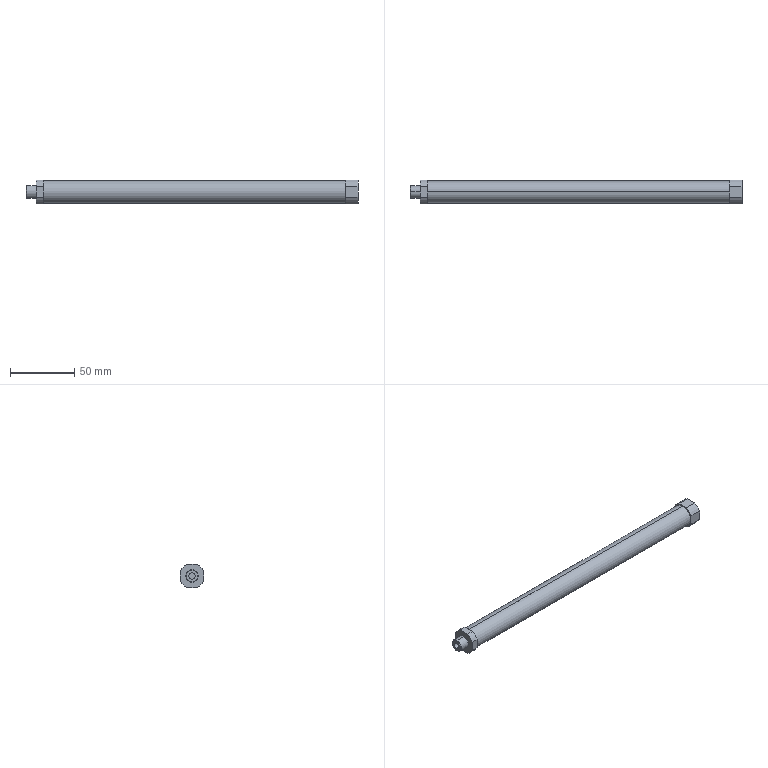Part | SolidWorks | features Chamfer 2, HoleWzd 2, ICE 2, Extrusion 1, Revolution 1 | 1 solid | 39 faces | box 259 x 18.3 x 18.3 mm | volume 34694 mm3 | cylinder 18 | plane 15 | cone 6 | commonest cylinder face diameters 20 x8 4.134 x2 5 x2 10 x2 16 x2 17.4 x2
STEP:
#1=CARTESIAN_POINT('',(246.,8.717,-2.067));
#2=VERTEX_POINT('',#1);
#3=CARTESIAN_POINT('',(246.,8.717,2.067));
#4=VERTEX_POINT('',#3);
#5=CARTESIAN_POINT('',(246.,8.717,0.));
#6=DIRECTION('',(0.,1.,0.));
#7=DIRECTION('',(0.,0.,1.));
#8=AXIS2_PLACEMENT_3D('',#5,#6,#7);
#9=CIRCLE('',#8,2.067);
#10=EDGE_CURVE('',#2,#4,#9,.T.);
#11=ORIENTED_EDGE('',*,*,#10,.F.);
#12=CARTESIAN_POINT('',(246.,9.15,-2.5));
#13=VERTEX_POINT('',#12);
#14=CARTESIAN_POINT('',(246.,8.717,-2.067));
#15=DIRECTION('',(0.,0.7071,-0.7071));
#16=VECTOR('',#15,1000.);
#17=LINE('',#14,#16);
#18=EDGE_CURVE('',#2,#13,#17,.T.);
#19=ORIENTED_EDGE('',*,*,#18,.T.);
#20=CARTESIAN_POINT('',(246.,9.15,2.5));
#21=VERTEX_POINT('',#20);
#22=CARTESIAN_POINT('',(246.,9.15,0.));
#23=DIRECTION('',(0.,-1.,0.));
#24=DIRECTION('',(0.,0.,1.));
#25=AXIS2_PLACEMENT_3D('',#22,#23,#24);
#26=CIRCLE('',#25,2.5);
#27=EDGE_CURVE('',#21,#13,#26,.T.);
#28=ORIENTED_EDGE('',*,*,#27,.F.);
#29=CARTESIAN_POINT('',(246.,8.717,2.067));
#30=DIRECTION('',(0.,0.7071,0.7071));
#31=VECTOR('',#30,1000.);
#32=LINE('',#29,#31);
#33=EDGE_CURVE('',#4,#21,#32,.T.);
#34=ORIENTED_EDGE('',*,*,#33,.F.);
#35=EDGE_LOOP('',(#11,#19,#28,#34));
#36=FACE_OUTER_BOUND('',#35,.T.);
#37=CARTESIAN_POINT('',(246.,8.717,0.));
#38=DIRECTION('',(0.,1.,0.));
#39=DIRECTION('',(0.,0.,1.));
#40=AXIS2_PLACEMENT_3D('',#37,#38,#39);
#41=CONICAL_SURFACE('',#40,2.067,0.7854);
#42=ADVANCED_FACE('',(#36),#41,.F.);
#43=CARTESIAN_POINT('',(-8.,0.,4.459));
#44=VERTEX_POINT('',#43);
#45=CARTESIAN_POINT('',(-8.,0.,-4.459));
#46=VERTEX_POINT('',#45);
#47=CARTESIAN_POINT('',(-8.,0.,0.));
#48=DIRECTION('',(-1.,0.,0.));
#49=DIRECTION('',(0.,0.,1.));
#50=AXIS2_PLACEMENT_3D('',#47,#48,#49);
#51=CIRCLE('',#50,4.459);
#52=EDGE_CURVE('',#44,#46,#51,.T.);
#53=ORIENTED_EDGE('',*,*,#52,.F.);
#54=CARTESIAN_POINT('',(-7.459,0.,5.));
#55=VERTEX_POINT('',#54);
#56=CARTESIAN_POINT('',(-7.459,0.,5.));
#57=DIRECTION('',(0.7071,0.,0.7071));
#58=VECTOR('',#57,1000.);
#59=LINE('',#56,#58);
#60=EDGE_CURVE('',#44,#55,#59,.T.);
#61=ORIENTED_EDGE('',*,*,#60,.T.);
#62=CARTESIAN_POINT('',(-7.459,0.,-5.));
#63=VERTEX_POINT('',#62);
#64=CARTESIAN_POINT('',(-7.459,0.,0.));
#65=DIRECTION('',(1.,0.,0.));
#66=DIRECTION('',(0.,0.,1.));
#67=AXIS2_PLACEMENT_3D('',#64,#65,#66);
#68=CIRCLE('',#67,5.);
#69=EDGE_CURVE('',#63,#55,#68,.T.);
#70=ORIENTED_EDGE('',*,*,#69,.F.);
#71=CARTESIAN_POINT('',(-7.459,0.,-5.));
#72=DIRECTION('',(0.7071,0.,-0.7071));
#73=VECTOR('',#72,1000.);
#74=LINE('',#71,#73);
#75=EDGE_CURVE('',#46,#63,#74,.T.);
#76=ORIENTED_EDGE('',*,*,#75,.F.);
#77=EDGE_LOOP('',(#53,#61,#70,#76));
#78=FACE_OUTER_BOUND('',#77,.T.);
#79=CARTESIAN_POINT('',(-7.459,0.,0.));
#80=DIRECTION('',(1.,0.,0.));
#81=DIRECTION('',(0.,0.,-1.));
#82=AXIS2_PLACEMENT_3D('',#79,#80,#81);
#83=CONICAL_SURFACE('',#82,5.,0.7854);
#84=ADVANCED_FACE('',(#78),#83,.T.);
#85=CARTESIAN_POINT('',(5.5,0.,-2.5));
#86=VERTEX_POINT('',#85);
#87=CARTESIAN_POINT('',(5.5,0.,2.5));
#88=VERTEX_POINT('',#87);
#89=CARTESIAN_POINT('',(5.5,0.,0.));
#90=DIRECTION('',(-1.,0.,0.));
#91=DIRECTION('',(0.,0.,1.));
#92=AXIS2_PLACEMENT_3D('',#89,#90,#91);
#93=CIRCLE('',#92,2.5);
#94=EDGE_CURVE('',#86,#88,#93,.T.);
#95=ORIENTED_EDGE('',*,*,#94,.F.);
#96=CARTESIAN_POINT('',(-8.,0.,-2.5));
#97=VERTEX_POINT('',#96);
#98=CARTESIAN_POINT('',(-8.,0.,-2.5));
#99=DIRECTION('',(-1.,0.,0.));
#100=VECTOR('',#99,1000.);
#101=LINE('',#98,#100);
#102=EDGE_CURVE('',#86,#97,#101,.T.);
#103=ORIENTED_EDGE('',*,*,#102,.T.);
#104=CARTESIAN_POINT('',(-8.,0.,2.5));
#105=VERTEX_POINT('',#104);
#106=CARTESIAN_POINT('',(-8.,0.,0.));
#107=DIRECTION('',(-1.,0.,0.));
#108=DIRECTION('',(0.,0.,1.));
#109=AXIS2_PLACEMENT_3D('',#106,#107,#108);
#110=CIRCLE('',#109,2.5);
#111=EDGE_CURVE('',#97,#105,#110,.T.);
#112=ORIENTED_EDGE('',*,*,#111,.T.);
#113=CARTESIAN_POINT('',(-8.,0.,2.5));
#114=DIRECTION('',(-1.,0.,0.));
#115=VECTOR('',#114,1000.);
#116=LINE('',#113,#115);
#117=EDGE_CURVE('',#88,#105,#116,.T.);
#118=ORIENTED_EDGE('',*,*,#117,.F.);
#119=EDGE_LOOP('',(#95,#103,#112,#118));
#120=FACE_OUTER_BOUND('',#119,.T.);
#121=CARTESIAN_POINT('',(-8.,0.,0.));
#122=DIRECTION('',(-1.,0.,0.));
#123=DIRECTION('',(0.,0.,1.));
#124=AXIS2_PLACEMENT_3D('',#121,#122,#123);
#125=CYLINDRICAL_SURFACE('',#124,2.5);
#126=ADVANCED_FACE('',(#120),#125,.F.);
#127=CARTESIAN_POINT('',(135.5,0.,-8.));
#128=VERTEX_POINT('',#127);
#129=CARTESIAN_POINT('',(135.5,0.,8.));
#130=VERTEX_POINT('',#129);
#131=CARTESIAN_POINT('',(135.5,0.,0.));
#132=DIRECTION('',(-1.,0.,0.));
#133=DIRECTION('',(0.,0.,1.));
#134=AXIS2_PLACEMENT_3D('',#131,#132,#133);
#135=CIRCLE('',#134,8.);
#136=EDGE_CURVE('',#128,#130,#135,.T.);
#137=ORIENTED_EDGE('',*,*,#136,.F.);
#138=CARTESIAN_POINT('',(5.5,0.,-8.));
#139=VERTEX_POINT('',#138);
#140=CARTESIAN_POINT('',(-8.,0.,-8.));
#141=DIRECTION('',(-1.,0.,0.));
#142=VECTOR('',#141,1000.);
#143=LINE('',#140,#142);
#144=EDGE_CURVE('',#128,#139,#143,.T.);
#145=ORIENTED_EDGE('',*,*,#144,.T.);
#146=CARTESIAN_POINT('',(5.5,0.,8.));
#147=VERTEX_POINT('',#146);
#148=CARTESIAN_POINT('',(5.5,0.,0.));
#149=DIRECTION('',(-1.,0.,0.));
#150=DIRECTION('',(0.,0.,1.));
#151=AXIS2_PLACEMENT_3D('',#148,#149,#150);
#152=CIRCLE('',#151,8.);
#153=EDGE_CURVE('',#139,#147,#152,.T.);
#154=ORIENTED_EDGE('',*,*,#153,.T.);
#155=CARTESIAN_POINT('',(-8.,0.,8.));
#156=DIRECTION('',(-1.,0.,0.));
#157=VECTOR('',#156,1000.);
#158=LINE('',#155,#157);
#159=EDGE_CURVE('',#130,#147,#158,.T.);
#160=ORIENTED_EDGE('',*,*,#159,.F.);
#161=EDGE_LOOP('',(#137,#145,#154,#160));
#162=FACE_OUTER_BOUND('',#161,.T.);
#163=CARTESIAN_POINT('',(-8.,0.,0.));
#164=DIRECTION('',(-1.,0.,0.));
#165=DIRECTION('',(0.,0.,1.));
#166=AXIS2_PLACEMENT_3D('',#163,#164,#165);
#167=CYLINDRICAL_SURFACE('',#166,8.);
#168=ADVANCED_FACE('',(#162),#167,.F.);
#169=CARTESIAN_POINT('',(246.,3.65,-2.067));
#170=VERTEX_POINT('',#169);
#171=CARTESIAN_POINT('',(246.,3.65,2.067));
#172=VERTEX_POINT('',#171);
#173=CARTESIAN_POINT('',(246.,3.65,0.));
#174=DIRECTION('',(0.,1.,0.));
#175=DIRECTION('',(0.,0.,1.));
#176=AXIS2_PLACEMENT_3D('',#173,#174,#175);
#177=CIRCLE('',#176,2.067);
#178=EDGE_CURVE('',#170,#172,#177,.T.);
#179=ORIENTED_EDGE('',*,*,#178,.F.);
#180=CARTESIAN_POINT('',(246.,9.15,-2.067));
#181=DIRECTION('',(0.,1.,0.));
#182=VECTOR('',#181,1000.);
#183=LINE('',#180,#182);
#184=EDGE_CURVE('',#170,#2,#183,.T.);
#185=ORIENTED_EDGE('',*,*,#184,.T.);
#186=ORIENTED_EDGE('',*,*,#10,.T.);
#187=CARTESIAN_POINT('',(246.,9.15,2.067));
#188=DIRECTION('',(0.,1.,0.));
#189=VECTOR('',#188,1000.);
#190=LINE('',#187,#189);
#191=EDGE_CURVE('',#172,#4,#190,.T.);
#192=ORIENTED_EDGE('',*,*,#191,.F.);
#193=EDGE_LOOP('',(#179,#185,#186,#192));
#194=FACE_OUTER_BOUND('',#193,.T.);
#195=CARTESIAN_POINT('',(246.,9.15,0.));
#196=DIRECTION('',(0.,1.,0.));
#197=DIRECTION('',(0.,0.,1.));
#198=AXIS2_PLACEMENT_3D('',#195,#196,#197);
#199=CYLINDRICAL_SURFACE('',#198,2.067);
#200=ADVANCED_FACE('',(#194),#199,.F.);
#201=CARTESIAN_POINT('',(246.,2.457,0.));
#202=VERTEX_POINT('',#201);
#203=CARTESIAN_POINT('',(246.,3.65,2.067));
#204=DIRECTION('',(0.,0.5,0.866));
#205=VECTOR('',#204,1000.);
#206=LINE('',#203,#205);
#207=EDGE_CURVE('',#202,#172,#206,.T.);
#208=ORIENTED_EDGE('',*,*,#207,.F.);
#209=CARTESIAN_POINT('',(246.,3.65,-2.067));
#210=DIRECTION('',(0.,0.5,-0.866));
#211=VECTOR('',#210,1000.);
#212=LINE('',#209,#211);
#213=EDGE_CURVE('',#202,#170,#212,.T.);
#214=ORIENTED_EDGE('',*,*,#213,.T.);
#215=ORIENTED_EDGE('',*,*,#178,.T.);
#216=EDGE_LOOP('',(#208,#214,#215));
#217=FACE_OUTER_BOUND('',#216,.T.);
#218=CARTESIAN_POINT('',(246.,3.65,0.));
#219=DIRECTION('',(0.,1.,0.));
#220=DIRECTION('',(0.,0.,1.));
#221=AXIS2_PLACEMENT_3D('',#218,#219,#220);
#222=CONICAL_SURFACE('',#221,2.067,1.047);
#223=ADVANCED_FACE('',(#217),#222,.F.);
#224=ORIENTED_EDGE('',*,*,#69,.T.);
#225=CARTESIAN_POINT('',(0.,0.,5.));
#226=VERTEX_POINT('',#225);
#227=CARTESIAN_POINT('',(-8.,0.,5.));
#228=DIRECTION('',(1.,0.,0.));
#229=VECTOR('',#228,1000.);
#230=LINE('',#227,#229);
#231=EDGE_CURVE('',#55,#226,#230,.T.);
#232=ORIENTED_EDGE('',*,*,#231,.T.);
#233=CARTESIAN_POINT('',(0.,0.,-5.));
#234=VERTEX_POINT('',#233);
#235=CARTESIAN_POINT('',(0.,0.,0.));
#236=DIRECTION('',(-1.,0.,0.));
#237=DIRECTION('',(0.,0.,1.));
#238=AXIS2_PLACEMENT_3D('',#235,#236,#237);
#239=CIRCLE('',#238,5.);
#240=EDGE_CURVE('',#226,#234,#239,.T.);
#241=ORIENTED_EDGE('',*,*,#240,.T.);
#242=CARTESIAN_POINT('',(-8.,0.,-5.));
#243=DIRECTION('',(1.,0.,0.));
#244=VECTOR('',#243,1000.);
#245=LINE('',#242,#244);
#246=EDGE_CURVE('',#63,#234,#245,.T.);
#247=ORIENTED_EDGE('',*,*,#246,.F.);
#248=EDGE_LOOP('',(#224,#232,#241,#247));
#249=FACE_OUTER_BOUND('',#248,.T.);
#250=CARTESIAN_POINT('',(-8.,0.,0.));
#251=DIRECTION('',(1.,0.,0.));
#252=DIRECTION('',(0.,0.,-1.));
#253=AXIS2_PLACEMENT_3D('',#250,#251,#252);
#254=CYLINDRICAL_SURFACE('',#253,5.);
#255=ADVANCED_FACE('',(#249),#254,.T.);
#256=CARTESIAN_POINT('',(241.5,0.,-8.7));
#257=VERTEX_POINT('',#256);
#258=CARTESIAN_POINT('',(241.5,0.,8.7));
#259=VERTEX_POINT('',#258);
#260=CARTESIAN_POINT('',(241.5,0.,0.));
#261=DIRECTION('',(1.,0.,0.));
#262=DIRECTION('',(0.,0.,-1.));
#263=AXIS2_PLACEMENT_3D('',#260,#261,#262);
#264=CIRCLE('',#263,8.7);
#265=EDGE_CURVE('',#257,#259,#264,.T.);
#266=ORIENTED_EDGE('',*,*,#265,.F.);
#267=CARTESIAN_POINT('',(5.5,0.,-8.7));
#268=VERTEX_POINT('',#267);
#269=CARTESIAN_POINT('',(241.5,0.,-8.7));
#270=DIRECTION('',(-1.,0.,0.));
#271=VECTOR('',#270,1000.);
#272=LINE('',#269,#271);
#273=EDGE_CURVE('',#257,#268,#272,.T.);
#274=ORIENTED_EDGE('',*,*,#273,.T.);
#275=CARTESIAN_POINT('',(5.5,0.,8.7));
#276=VERTEX_POINT('',#275);
#277=CARTESIAN_POINT('',(5.5,0.,0.));
#278=DIRECTION('',(1.,0.,0.));
#279=DIRECTION('',(0.,0.,1.));
#280=AXIS2_PLACEMENT_3D('',#277,#278,#279);
#281=CIRCLE('',#280,8.7);
#282=EDGE_CURVE('',#268,#276,#281,.T.);
#283=ORIENTED_EDGE('',*,*,#282,.T.);
#284=CARTESIAN_POINT('',(241.5,0.,8.7));
#285=DIRECTION('',(-1.,0.,0.));
#286=VECTOR('',#285,1000.);
#287=LINE('',#284,#286);
#288=EDGE_CURVE('',#259,#276,#287,.T.);
#289=ORIENTED_EDGE('',*,*,#288,.F.);
#290=EDGE_LOOP('',(#266,#274,#283,#289));
#291=FACE_OUTER_BOUND('',#290,.T.);
#292=CARTESIAN_POINT('',(241.5,0.,0.));
#293=DIRECTION('',(-1.,0.,0.));
#294=DIRECTION('',(0.,0.,1.));
#295=AXIS2_PLACEMENT_3D('',#292,#293,#294);
#296=CYLINDRICAL_SURFACE('',#295,8.7);
#297=ADVANCED_FACE('',(#291),#296,.T.);
#298=CARTESIAN_POINT('',(5.5,-9.15,4.035));
#299=VERTEX_POINT('',#298);
#300=CARTESIAN_POINT('',(5.5,-4.035,9.15));
#301=VERTEX_POINT('',#300);
#302=CARTESIAN_POINT('',(5.5,0.,0.));
#303=DIRECTION('',(-1.,0.,0.));
#304=DIRECTION('',(0.,0.,1.));
#305=AXIS2_PLACEMENT_3D('',#302,#303,#304);
#306=CIRCLE('',#305,10.);
#307=EDGE_CURVE('',#299,#301,#306,.T.);
#308=ORIENTED_EDGE('',*,*,#307,.F.);
#309=CARTESIAN_POINT('',(5.5,-9.15,-4.035));
#310=VERTEX_POINT('',#309);
#311=CARTESIAN_POINT('',(5.5,-9.15,-4.035));
#312=DIRECTION('',(0.,0.,1.));
#313=VECTOR('',#312,1000.);
#314=LINE('',#311,#313);
#315=EDGE_CURVE('',#310,#299,#314,.T.);
#316=ORIENTED_EDGE('',*,*,#315,.F.);
#317=CARTESIAN_POINT('',(5.5,-4.035,-9.15));
#318=VERTEX_POINT('',#317);
#319=CARTESIAN_POINT('',(5.5,0.,0.));
#320=DIRECTION('',(-1.,0.,0.));
#321=DIRECTION('',(0.,0.,1.));
#322=AXIS2_PLACEMENT_3D('',#319,#320,#321);
#323=CIRCLE('',#322,10.);
#324=EDGE_CURVE('',#318,#310,#323,.T.);
#325=ORIENTED_EDGE('',*,*,#324,.F.);
#326=CARTESIAN_POINT('',(5.5,4.035,-9.15));
#327=VERTEX_POINT('',#326);
#328=CARTESIAN_POINT('',(5.5,4.035,-9.15));
#329=DIRECTION('',(0.,-1.,0.));
#330=VECTOR('',#329,1000.);
#331=LINE('',#328,#330);
#332=EDGE_CURVE('',#327,#318,#331,.T.);
#333=ORIENTED_EDGE('',*,*,#332,.F.);
#334=CARTESIAN_POINT('',(5.5,9.15,-4.035));
#335=VERTEX_POINT('',#334);
#336=CARTESIAN_POINT('',(5.5,0.,0.));
#337=DIRECTION('',(-1.,0.,0.));
#338=DIRECTION('',(0.,0.,1.));
#339=AXIS2_PLACEMENT_3D('',#336,#337,#338);
#340=CIRCLE('',#339,10.);
#341=EDGE_CURVE('',#335,#327,#340,.T.);
#342=ORIENTED_EDGE('',*,*,#341,.F.);
#343=CARTESIAN_POINT('',(5.5,9.15,4.035));
#344=VERTEX_POINT('',#343);
#345=CARTESIAN_POINT('',(5.5,9.15,4.035));
#346=DIRECTION('',(0.,0.,-1.));
#347=VECTOR('',#346,1000.);
#348=LINE('',#345,#347);
#349=EDGE_CURVE('',#344,#335,#348,.T.);
#350=ORIENTED_EDGE('',*,*,#349,.F.);
#351=CARTESIAN_POINT('',(5.5,4.035,9.15));
#352=VERTEX_POINT('',#351);
#353=CARTESIAN_POINT('',(5.5,0.,0.));
#354=DIRECTION('',(-1.,0.,0.));
#355=DIRECTION('',(0.,0.,1.));
#356=AXIS2_PLACEMENT_3D('',#353,#354,#355);
#357=CIRCLE('',#356,10.);
#358=EDGE_CURVE('',#352,#344,#357,.T.);
#359=ORIENTED_EDGE('',*,*,#358,.F.);
#360=CARTESIAN_POINT('',(5.5,-4.035,9.15));
#361=DIRECTION('',(0.,1.,0.));
#362=VECTOR('',#361,1000.);
#363=LINE('',#360,#362);
#364=EDGE_CURVE('',#301,#352,#363,.T.);
#365=ORIENTED_EDGE('',*,*,#364,.F.);
#366=EDGE_LOOP('',(#308,#316,#325,#333,#342,#350,#359,#365));
#367=FACE_OUTER_BOUND('',#366,.T.);
#368=CARTESIAN_POINT('',(5.5,0.,0.));
#369=DIRECTION('',(1.,0.,0.));
#370=DIRECTION('',(0.,0.,1.));
#371=AXIS2_PLACEMENT_3D('',#368,#369,#370);
#372=CIRCLE('',#371,8.7);
#373=EDGE_CURVE('',#276,#268,#372,.T.);
#374=ORIENTED_EDGE('',*,*,#373,.F.);
#375=ORIENTED_EDGE('',*,*,#282,.F.);
#376=EDGE_LOOP('',(#374,#375));
#377=FACE_BOUND('',#376,.T.);
#378=CARTESIAN_POINT('',(5.5,0.,0.));
#379=DIRECTION('',(-1.,0.,0.));
#380=DIRECTION('',(0.,0.,1.));
#381=AXIS2_PLACEMENT_3D('',#378,#379,#380);
#382=PLANE('',#381);
#383=ADVANCED_FACE('',(#367,#377),#382,.F.);
#384=CARTESIAN_POINT('',(0.,-9.15,4.035));
#385=VERTEX_POINT('',#384);
#386=CARTESIAN_POINT('',(0.,-4.035,9.15));
#387=VERTEX_POINT('',#386);
#388=CARTESIAN_POINT('',(0.,0.,0.));
#389=DIRECTION('',(-1.,0.,0.));
#390=DIRECTION('',(0.,0.,1.));
#391=AXIS2_PLACEMENT_3D('',#388,#389,#390);
#392=CIRCLE('',#391,10.);
#393=EDGE_CURVE('',#385,#387,#392,.T.);
#394=ORIENTED_EDGE('',*,*,#393,.F.);
#395=CARTESIAN_POINT('',(5.5,-9.15,4.035));
#396=DIRECTION('',(-1.,0.,0.));
#397=VECTOR('',#396,1000.);
#398=LINE('',#395,#397);
#399=EDGE_CURVE('',#299,#385,#398,.T.);
#400=ORIENTED_EDGE('',*,*,#399,.F.);
#401=ORIENTED_EDGE('',*,*,#307,.T.);
#402=CARTESIAN_POINT('',(5.5,-4.035,9.15));
#403=DIRECTION('',(-1.,0.,0.));
#404=VECTOR('',#403,1000.);
#405=LINE('',#402,#404);
#406=EDGE_CURVE('',#301,#387,#405,.T.);
#407=ORIENTED_EDGE('',*,*,#406,.T.);
#408=EDGE_LOOP('',(#394,#400,#401,#407));
#409=FACE_OUTER_BOUND('',#408,.T.);
#410=CARTESIAN_POINT('',(5.5,0.,0.));
#411=DIRECTION('',(-1.,0.,0.));
#412=DIRECTION('',(0.,0.,1.));
#413=AXIS2_PLACEMENT_3D('',#410,#411,#412);
#414=CYLINDRICAL_SURFACE('',#413,10.);
#415=ADVANCED_FACE('',(#409),#414,.T.);
#416=CARTESIAN_POINT('',(0.,-9.15,-4.035));
#417=VERTEX_POINT('',#416);
#418=CARTESIAN_POINT('',(0.,-9.15,-4.035));
#419=DIRECTION('',(0.,0.,1.));
#420=VECTOR('',#419,1000.);
#421=LINE('',#418,#420);
#422=EDGE_CURVE('',#417,#385,#421,.T.);
#423=ORIENTED_EDGE('',*,*,#422,.F.);
#424=CARTESIAN_POINT('',(5.5,-9.15,-4.035));
#425=DIRECTION('',(-1.,0.,0.));
#426=VECTOR('',#425,1000.);
#427=LINE('',#424,#426);
#428=EDGE_CURVE('',#310,#417,#427,.T.);
#429=ORIENTED_EDGE('',*,*,#428,.F.);
#430=ORIENTED_EDGE('',*,*,#315,.T.);
#431=ORIENTED_EDGE('',*,*,#399,.T.);
#432=EDGE_LOOP('',(#423,#429,#430,#431));
#433=FACE_OUTER_BOUND('',#432,.T.);
#434=CARTESIAN_POINT('',(5.5,-9.15,-4.035));
#435=DIRECTION('',(0.,-1.,0.));
#436=DIRECTION('',(0.,0.,-1.));
#437=AXIS2_PLACEMENT_3D('',#434,#435,#436);
#438=PLANE('',#437);
#439=ADVANCED_FACE('',(#433),#438,.T.);
#440=CARTESIAN_POINT('',(0.,-4.035,-9.15));
#441=VERTEX_POINT('',#440);
#442=CARTESIAN_POINT('',(0.,0.,0.));
#443=DIRECTION('',(-1.,0.,0.));
#444=DIRECTION('',(0.,0.,1.));
#445=AXIS2_PLACEMENT_3D('',#442,#443,#444);
#446=CIRCLE('',#445,10.);
#447=EDGE_CURVE('',#441,#417,#446,.T.);
#448=ORIENTED_EDGE('',*,*,#447,.F.);
#449=CARTESIAN_POINT('',(5.5,-4.035,-9.15));
#450=DIRECTION('',(-1.,0.,0.));
#451=VECTOR('',#450,1000.);
#452=LINE('',#449,#451);
#453=EDGE_CURVE('',#318,#441,#452,.T.);
#454=ORIENTED_EDGE('',*,*,#453,.F.);
#455=ORIENTED_EDGE('',*,*,#324,.T.);
#456=ORIENTED_EDGE('',*,*,#428,.T.);
#457=EDGE_LOOP('',(#448,#454,#455,#456));
#458=FACE_OUTER_BOUND('',#457,.T.);
#459=CARTESIAN_POINT('',(5.5,0.,0.));
#460=DIRECTION('',(-1.,0.,0.));
#461=DIRECTION('',(0.,0.,1.));
#462=AXIS2_PLACEMENT_3D('',#459,#460,#461);
#463=CYLINDRICAL_SURFACE('',#462,10.);
#464=ADVANCED_FACE('',(#458),#463,.T.);
#465=CARTESIAN_POINT('',(0.,4.035,-9.15));
#466=VERTEX_POINT('',#465);
#467=CARTESIAN_POINT('',(0.,4.035,-9.15));
#468=DIRECTION('',(0.,-1.,0.));
#469=VECTOR('',#468,1000.);
#470=LINE('',#467,#469);
#471=EDGE_CURVE('',#466,#441,#470,.T.);
#472=ORIENTED_EDGE('',*,*,#471,.F.);
#473=CARTESIAN_POINT('',(5.5,4.035,-9.15));
#474=DIRECTION('',(-1.,0.,0.));
#475=VECTOR('',#474,1000.);
#476=LINE('',#473,#475);
#477=EDGE_CURVE('',#327,#466,#476,.T.);
#478=ORIENTED_EDGE('',*,*,#477,.F.);
#479=ORIENTED_EDGE('',*,*,#332,.T.);
#480=ORIENTED_EDGE('',*,*,#453,.T.);
#481=EDGE_LOOP('',(#472,#478,#479,#480));
#482=FACE_OUTER_BOUND('',#481,.T.);
#483=CARTESIAN_POINT('',(5.5,4.035,-9.15));
#484=DIRECTION('',(0.,0.,-1.));
#485=DIRECTION('',(0.,1.,0.));
#486=AXIS2_PLACEMENT_3D('',#483,#484,#485);
#487=PLANE('',#486);
#488=ADVANCED_FACE('',(#482),#487,.T.);
#489=CARTESIAN_POINT('',(0.,9.15,-4.035));
#490=VERTEX_POINT('',#489);
#491=CARTESIAN_POINT('',(0.,0.,0.));
#492=DIRECTION('',(-1.,0.,0.));
#493=DIRECTION('',(0.,0.,1.));
#494=AXIS2_PLACEMENT_3D('',#491,#492,#493);
#495=CIRCLE('',#494,10.);
#496=EDGE_CURVE('',#490,#466,#495,.T.);
#497=ORIENTED_EDGE('',*,*,#496,.F.);
#498=CARTESIAN_POINT('',(5.5,9.15,-4.035));
#499=DIRECTION('',(-1.,0.,0.));
#500=VECTOR('',#499,1000.);
#501=LINE('',#498,#500);
#502=EDGE_CURVE('',#335,#490,#501,.T.);
#503=ORIENTED_EDGE('',*,*,#502,.F.);
#504=ORIENTED_EDGE('',*,*,#341,.T.);
#505=ORIENTED_EDGE('',*,*,#477,.T.);
#506=EDGE_LOOP('',(#497,#503,#504,#505));
#507=FACE_OUTER_BOUND('',#506,.T.);
#508=CARTESIAN_POINT('',(5.5,0.,0.));
#509=DIRECTION('',(-1.,0.,0.));
#510=DIRECTION('',(0.,0.,1.));
#511=AXIS2_PLACEMENT_3D('',#508,#509,#510);
#512=CYLINDRICAL_SURFACE('',#511,10.);
#513=ADVANCED_FACE('',(#507),#512,.T.);
#514=CARTESIAN_POINT('',(0.,9.15,4.035));
#515=VERTEX_POINT('',#514);
#516=CARTESIAN_POINT('',(0.,9.15,4.035));
#517=DIRECTION('',(0.,0.,-1.));
#518=VECTOR('',#517,1000.);
#519=LINE('',#516,#518);
#520=EDGE_CURVE('',#515,#490,#519,.T.);
#521=ORIENTED_EDGE('',*,*,#520,.F.);
#522=CARTESIAN_POINT('',(5.5,9.15,4.035));
#523=DIRECTION('',(-1.,0.,0.));
#524=VECTOR('',#523,1000.);
#525=LINE('',#522,#524);
#526=EDGE_CURVE('',#344,#515,#525,.T.);
#527=ORIENTED_EDGE('',*,*,#526,.F.);
#528=ORIENTED_EDGE('',*,*,#349,.T.);
#529=ORIENTED_EDGE('',*,*,#502,.T.);
#530=EDGE_LOOP('',(#521,#527,#528,#529));
#531=FACE_OUTER_BOUND('',#530,.T.);
#532=CARTESIAN_POINT('',(5.5,9.15,4.035));
#533=DIRECTION('',(0.,1.,0.));
#534=DIRECTION('',(0.,0.,1.));
#535=AXIS2_PLACEMENT_3D('',#532,#533,#534);
#536=PLANE('',#535);
#537=ADVANCED_FACE('',(#531),#536,.T.);
#538=CARTESIAN_POINT('',(0.,4.035,9.15));
#539=VERTEX_POINT('',#538);
#540=CARTESIAN_POINT('',(0.,0.,0.));
#541=DIRECTION('',(-1.,0.,0.));
#542=DIRECTION('',(0.,0.,1.));
#543=AXIS2_PLACEMENT_3D('',#540,#541,#542);
#544=CIRCLE('',#543,10.);
#545=EDGE_CURVE('',#539,#515,#544,.T.);
#546=ORIENTED_EDGE('',*,*,#545,.F.);
#547=CARTESIAN_POINT('',(5.5,4.035,9.15));
#548=DIRECTION('',(-1.,0.,0.));
#549=VECTOR('',#548,1000.);
#550=LINE('',#547,#549);
#551=EDGE_CURVE('',#352,#539,#550,.T.);
#552=ORIENTED_EDGE('',*,*,#551,.F.);
#553=ORIENTED_EDGE('',*,*,#358,.T.);
#554=ORIENTED_EDGE('',*,*,#526,.T.);
#555=EDGE_LOOP('',(#546,#552,#553,#554));
#556=FACE_OUTER_BOUND('',#555,.T.);
#557=CARTESIAN_POINT('',(5.5,0.,0.));
#558=DIRECTION('',(-1.,0.,0.));
#559=DIRECTION('',(0.,0.,1.));
#560=AXIS2_PLACEMENT_3D('',#557,#558,#559);
#561=CYLINDRICAL_SURFACE('',#560,10.);
#562=ADVANCED_FACE('',(#556),#561,.T.);
#563=CARTESIAN_POINT('',(0.,-4.035,9.15));
#564=DIRECTION('',(0.,1.,0.));
#565=VECTOR('',#564,1000.);
#566=LINE('',#563,#565);
#567=EDGE_CURVE('',#387,#539,#566,.T.);
#568=ORIENTED_EDGE('',*,*,#567,.F.);
#569=ORIENTED_EDGE('',*,*,#406,.F.);
#570=ORIENTED_EDGE('',*,*,#364,.T.);
#571=ORIENTED_EDGE('',*,*,#551,.T.);
#572=EDGE_LOOP('',(#568,#569,#570,#571));
#573=FACE_OUTER_BOUND('',#572,.T.);
#574=CARTESIAN_POINT('',(5.5,-4.035,9.15));
#575=DIRECTION('',(0.,0.,1.));
#576=DIRECTION('',(0.,-1.,0.));
#577=AXIS2_PLACEMENT_3D('',#574,#575,#576);
#578=PLANE('',#577);
#579=ADVANCED_FACE('',(#573),#578,.T.);
#580=CARTESIAN_POINT('',(0.,0.,0.));
#581=DIRECTION('',(-1.,0.,0.));
#582=DIRECTION('',(0.,0.,1.));
#583=AXIS2_PLACEMENT_3D('',#580,#581,#582);
#584=CIRCLE('',#583,5.);
#585=EDGE_CURVE('',#234,#226,#584,.T.);
#586=ORIENTED_EDGE('',*,*,#585,.F.);
#587=ORIENTED_EDGE('',*,*,#240,.F.);
#588=EDGE_LOOP('',(#586,#587));
#589=FACE_BOUND('',#588,.T.);
#590=ORIENTED_EDGE('',*,*,#393,.T.);
#591=ORIENTED_EDGE('',*,*,#567,.T.);
#592=ORIENTED_EDGE('',*,*,#545,.T.);
#593=ORIENTED_EDGE('',*,*,#520,.T.);
#594=ORIENTED_EDGE('',*,*,#496,.T.);
#595=ORIENTED_EDGE('',*,*,#471,.T.);
#596=ORIENTED_EDGE('',*,*,#447,.T.);
#597=ORIENTED_EDGE('',*,*,#422,.T.);
#598=EDGE_LOOP('',(#590,#591,#592,#593,#594,#595,#596,#597));
#599=FACE_OUTER_BOUND('',#598,.T.);
#600=CARTESIAN_POINT('',(0.,0.,0.));
#601=DIRECTION('',(-1.,0.,0.));
#602=DIRECTION('',(0.,0.,1.));
#603=AXIS2_PLACEMENT_3D('',#600,#601,#602);
#604=PLANE('',#603);
#605=ADVANCED_FACE('',(#589,#599),#604,.T.);
#606=ORIENTED_EDGE('',*,*,#273,.F.);
#607=CARTESIAN_POINT('',(241.5,0.,0.));
#608=DIRECTION('',(1.,0.,0.));
#609=DIRECTION('',(0.,0.,-1.));
#610=AXIS2_PLACEMENT_3D('',#607,#608,#609);
#611=CIRCLE('',#610,8.7);
#612=EDGE_CURVE('',#259,#257,#611,.T.);
#613=ORIENTED_EDGE('',*,*,#612,.F.);
#614=ORIENTED_EDGE('',*,*,#288,.T.);
#615=ORIENTED_EDGE('',*,*,#373,.T.);
#616=EDGE_LOOP('',(#606,#613,#614,#615));
#617=FACE_OUTER_BOUND('',#616,.T.);
#618=CARTESIAN_POINT('',(241.5,0.,0.));
#619=DIRECTION('',(-1.,0.,0.));
#620=DIRECTION('',(0.,0.,1.));
#621=AXIS2_PLACEMENT_3D('',#618,#619,#620);
#622=CYLINDRICAL_SURFACE('',#621,8.7);
#623=ADVANCED_FACE('',(#617),#622,.T.);
#624=CARTESIAN_POINT('',(241.5,4.035,9.15));
#625=VERTEX_POINT('',#624);
#626=CARTESIAN_POINT('',(241.5,9.15,4.035));
#627=VERTEX_POINT('',#626);
#628=CARTESIAN_POINT('',(241.5,0.,0.));
#629=DIRECTION('',(-1.,0.,0.));
#630=DIRECTION('',(0.,0.,1.));
#631=AXIS2_PLACEMENT_3D('',#628,#629,#630);
#632=CIRCLE('',#631,10.);
#633=EDGE_CURVE('',#625,#627,#632,.T.);
#634=ORIENTED_EDGE('',*,*,#633,.T.);
#635=CARTESIAN_POINT('',(241.5,9.15,-4.035));
#636=VERTEX_POINT('',#635);
#637=CARTESIAN_POINT('',(241.5,9.15,4.035));
#638=DIRECTION('',(0.,0.,-1.));
#639=VECTOR('',#638,1000.);
#640=LINE('',#637,#639);
#641=EDGE_CURVE('',#627,#636,#640,.T.);
#642=ORIENTED_EDGE('',*,*,#641,.T.);
#643=CARTESIAN_POINT('',(241.5,4.035,-9.15));
#644=VERTEX_POINT('',#643);
#645=CARTESIAN_POINT('',(241.5,0.,0.));
#646=DIRECTION('',(-1.,0.,0.));
#647=DIRECTION('',(0.,0.,1.));
#648=AXIS2_PLACEMENT_3D('',#645,#646,#647);
#649=CIRCLE('',#648,10.);
#650=EDGE_CURVE('',#636,#644,#649,.T.);
#651=ORIENTED_EDGE('',*,*,#650,.T.);
#652=CARTESIAN_POINT('',(241.5,-4.035,-9.15));
#653=VERTEX_POINT('',#652);
#654=CARTESIAN_POINT('',(241.5,4.035,-9.15));
#655=DIRECTION('',(0.,-1.,0.));
#656=VECTOR('',#655,1000.);
#657=LINE('',#654,#656);
#658=EDGE_CURVE('',#644,#653,#657,.T.);
#659=ORIENTED_EDGE('',*,*,#658,.T.);
#660=CARTESIAN_POINT('',(241.5,-9.15,-4.035));
#661=VERTEX_POINT('',#660);
#662=CARTESIAN_POINT('',(241.5,0.,0.));
#663=DIRECTION('',(-1.,0.,0.));
#664=DIRECTION('',(0.,0.,1.));
#665=AXIS2_PLACEMENT_3D('',#662,#663,#664);
#666=CIRCLE('',#665,10.);
#667=EDGE_CURVE('',#653,#661,#666,.T.);
#668=ORIENTED_EDGE('',*,*,#667,.T.);
#669=CARTESIAN_POINT('',(241.5,-9.15,4.035));
#670=VERTEX_POINT('',#669);
#671=CARTESIAN_POINT('',(241.5,-9.15,-4.035));
#672=DIRECTION('',(0.,0.,1.));
#673=VECTOR('',#672,1000.);
#674=LINE('',#671,#673);
#675=EDGE_CURVE('',#661,#670,#674,.T.);
#676=ORIENTED_EDGE('',*,*,#675,.T.);
#677=CARTESIAN_POINT('',(241.5,-4.035,9.15));
#678=VERTEX_POINT('',#677);
#679=CARTESIAN_POINT('',(241.5,0.,0.));
#680=DIRECTION('',(-1.,0.,0.));
#681=DIRECTION('',(0.,0.,1.));
#682=AXIS2_PLACEMENT_3D('',#679,#680,#681);
#683=CIRCLE('',#682,10.);
#684=EDGE_CURVE('',#670,#678,#683,.T.);
#685=ORIENTED_EDGE('',*,*,#684,.T.);
#686=CARTESIAN_POINT('',(241.5,-4.035,9.15));
#687=DIRECTION('',(0.,1.,0.));
#688=VECTOR('',#687,1000.);
#689=LINE('',#686,#688);
#690=EDGE_CURVE('',#678,#625,#689,.T.);
#691=ORIENTED_EDGE('',*,*,#690,.T.);
#692=EDGE_LOOP('',(#634,#642,#651,#659,#668,#676,#685,#691));
#693=FACE_OUTER_BOUND('',#692,.T.);
#694=ORIENTED_EDGE('',*,*,#612,.T.);
#695=ORIENTED_EDGE('',*,*,#265,.T.);
#696=EDGE_LOOP('',(#694,#695));
#697=FACE_BOUND('',#696,.T.);
#698=CARTESIAN_POINT('',(241.5,0.,0.));
#699=DIRECTION('',(-1.,0.,0.));
#700=DIRECTION('',(0.,0.,1.));
#701=AXIS2_PLACEMENT_3D('',#698,#699,#700);
#702=PLANE('',#701);
#703=ADVANCED_FACE('',(#693,#697),#702,.T.);
#704=ORIENTED_EDGE('',*,*,#633,.F.);
#705=CARTESIAN_POINT('',(251.,4.035,9.15));
#706=VERTEX_POINT('',#705);
#707=CARTESIAN_POINT('',(251.,4.035,9.15));
#708=DIRECTION('',(-1.,0.,0.));
#709=VECTOR('',#708,1000.);
#710=LINE('',#707,#709);
#711=EDGE_CURVE('',#706,#625,#710,.T.);
#712=ORIENTED_EDGE('',*,*,#711,.F.);
#713=CARTESIAN_POINT('',(251.,9.15,4.035));
#714=VERTEX_POINT('',#713);
#715=CARTESIAN_POINT('',(251.,0.,0.));
#716=DIRECTION('',(-1.,0.,0.));
#717=DIRECTION('',(0.,0.,1.));
#718=AXIS2_PLACEMENT_3D('',#715,#716,#717);
#719=CIRCLE('',#718,10.);
#720=EDGE_CURVE('',#706,#714,#719,.T.);
#721=ORIENTED_EDGE('',*,*,#720,.T.);
#722=CARTESIAN_POINT('',(251.,9.15,4.035));
#723=DIRECTION('',(-1.,0.,0.));
#724=VECTOR('',#723,1000.);
#725=LINE('',#722,#724);
#726=EDGE_CURVE('',#714,#627,#725,.T.);
#727=ORIENTED_EDGE('',*,*,#726,.T.);
#728=EDGE_LOOP('',(#704,#712,#721,#727));
#729=FACE_OUTER_BOUND('',#728,.T.);
#730=CARTESIAN_POINT('',(251.,0.,0.));
#731=DIRECTION('',(-1.,0.,0.));
#732=DIRECTION('',(0.,0.,1.));
#733=AXIS2_PLACEMENT_3D('',#730,#731,#732);
#734=CYLINDRICAL_SURFACE('',#733,10.);
#735=ADVANCED_FACE('',(#729),#734,.T.);
#736=ORIENTED_EDGE('',*,*,#690,.F.);
#737=CARTESIAN_POINT('',(251.,-4.035,9.15));
#738=VERTEX_POINT('',#737);
#739=CARTESIAN_POINT('',(251.,-4.035,9.15));
#740=DIRECTION('',(-1.,0.,0.));
#741=VECTOR('',#740,1000.);
#742=LINE('',#739,#741);
#743=EDGE_CURVE('',#738,#678,#742,.T.);
#744=ORIENTED_EDGE('',*,*,#743,.F.);
#745=CARTESIAN_POINT('',(251.,-4.035,9.15));
#746=DIRECTION('',(0.,1.,0.));
#747=VECTOR('',#746,1000.);
#748=LINE('',#745,#747);
#749=EDGE_CURVE('',#738,#706,#748,.T.);
#750=ORIENTED_EDGE('',*,*,#749,.T.);
#751=ORIENTED_EDGE('',*,*,#711,.T.);
#752=EDGE_LOOP('',(#736,#744,#750,#751));
#753=FACE_OUTER_BOUND('',#752,.T.);
#754=CARTESIAN_POINT('',(251.,-4.035,9.15));
#755=DIRECTION('',(0.,0.,1.));
#756=DIRECTION('',(1.,0.,0.));
#757=AXIS2_PLACEMENT_3D('',#754,#755,#756);
#758=PLANE('',#757);
#759=ADVANCED_FACE('',(#753),#758,.T.);
#760=ORIENTED_EDGE('',*,*,#684,.F.);
#761=CARTESIAN_POINT('',(251.,-9.15,4.035));
#762=VERTEX_POINT('',#761);
#763=CARTESIAN_POINT('',(251.,-9.15,4.035));
#764=DIRECTION('',(-1.,0.,0.));
#765=VECTOR('',#764,1000.);
#766=LINE('',#763,#765);
#767=EDGE_CURVE('',#762,#670,#766,.T.);
#768=ORIENTED_EDGE('',*,*,#767,.F.);
#769=CARTESIAN_POINT('',(251.,0.,0.));
#770=DIRECTION('',(-1.,0.,0.));
#771=DIRECTION('',(0.,0.,1.));
#772=AXIS2_PLACEMENT_3D('',#769,#770,#771);
#773=CIRCLE('',#772,10.);
#774=EDGE_CURVE('',#762,#738,#773,.T.);
#775=ORIENTED_EDGE('',*,*,#774,.T.);
#776=ORIENTED_EDGE('',*,*,#743,.T.);
#777=EDGE_LOOP('',(#760,#768,#775,#776));
#778=FACE_OUTER_BOUND('',#777,.T.);
#779=CARTESIAN_POINT('',(251.,0.,0.));
#780=DIRECTION('',(-1.,0.,0.));
#781=DIRECTION('',(0.,0.,1.));
#782=AXIS2_PLACEMENT_3D('',#779,#780,#781);
#783=CYLINDRICAL_SURFACE('',#782,10.);
#784=ADVANCED_FACE('',(#778),#783,.T.);
#785=ORIENTED_EDGE('',*,*,#675,.F.);
#786=CARTESIAN_POINT('',(251.,-9.15,-4.035));
#787=VERTEX_POINT('',#786);
#788=CARTESIAN_POINT('',(251.,-9.15,-4.035));
#789=DIRECTION('',(-1.,0.,0.));
#790=VECTOR('',#789,1000.);
#791=LINE('',#788,#790);
#792=EDGE_CURVE('',#787,#661,#791,.T.);
#793=ORIENTED_EDGE('',*,*,#792,.F.);
#794=CARTESIAN_POINT('',(251.,-9.15,-4.035));
#795=DIRECTION('',(0.,0.,1.));
#796=VECTOR('',#795,1000.);
#797=LINE('',#794,#796);
#798=EDGE_CURVE('',#787,#762,#797,.T.);
#799=ORIENTED_EDGE('',*,*,#798,.T.);
#800=ORIENTED_EDGE('',*,*,#767,.T.);
#801=EDGE_LOOP('',(#785,#793,#799,#800));
#802=FACE_OUTER_BOUND('',#801,.T.);
#803=CARTESIAN_POINT('',(251.,-9.15,-4.035));
#804=DIRECTION('',(0.,-1.,0.));
#805=DIRECTION('',(0.,0.,-1.));
#806=AXIS2_PLACEMENT_3D('',#803,#804,#805);
#807=PLANE('',#806);
#808=ADVANCED_FACE('',(#802),#807,.T.);
#809=ORIENTED_EDGE('',*,*,#667,.F.);
#810=CARTESIAN_POINT('',(251.,-4.035,-9.15));
#811=VERTEX_POINT('',#810);
#812=CARTESIAN_POINT('',(251.,-4.035,-9.15));
#813=DIRECTION('',(-1.,0.,0.));
#814=VECTOR('',#813,1000.);
#815=LINE('',#812,#814);
#816=EDGE_CURVE('',#811,#653,#815,.T.);
#817=ORIENTED_EDGE('',*,*,#816,.F.);
#818=CARTESIAN_POINT('',(251.,0.,0.));
#819=DIRECTION('',(-1.,0.,0.));
#820=DIRECTION('',(0.,0.,1.));
#821=AXIS2_PLACEMENT_3D('',#818,#819,#820);
#822=CIRCLE('',#821,10.);
#823=EDGE_CURVE('',#811,#787,#822,.T.);
#824=ORIENTED_EDGE('',*,*,#823,.T.);
#825=ORIENTED_EDGE('',*,*,#792,.T.);
#826=EDGE_LOOP('',(#809,#817,#824,#825));
#827=FACE_OUTER_BOUND('',#826,.T.);
#828=CARTESIAN_POINT('',(251.,0.,0.));
#829=DIRECTION('',(-1.,0.,0.));
#830=DIRECTION('',(0.,0.,1.));
#831=AXIS2_PLACEMENT_3D('',#828,#829,#830);
#832=CYLINDRICAL_SURFACE('',#831,10.);
#833=ADVANCED_FACE('',(#827),#832,.T.);
#834=ORIENTED_EDGE('',*,*,#658,.F.);
#835=CARTESIAN_POINT('',(251.,4.035,-9.15));
#836=VERTEX_POINT('',#835);
#837=CARTESIAN_POINT('',(251.,4.035,-9.15));
#838=DIRECTION('',(-1.,0.,0.));
#839=VECTOR('',#838,1000.);
#840=LINE('',#837,#839);
#841=EDGE_CURVE('',#836,#644,#840,.T.);
#842=ORIENTED_EDGE('',*,*,#841,.F.);
#843=CARTESIAN_POINT('',(251.,4.035,-9.15));
#844=DIRECTION('',(0.,-1.,0.));
#845=VECTOR('',#844,1000.);
#846=LINE('',#843,#845);
#847=EDGE_CURVE('',#836,#811,#846,.T.);
#848=ORIENTED_EDGE('',*,*,#847,.T.);
#849=ORIENTED_EDGE('',*,*,#816,.T.);
#850=EDGE_LOOP('',(#834,#842,#848,#849));
#851=FACE_OUTER_BOUND('',#850,.T.);
#852=CARTESIAN_POINT('',(251.,4.035,-9.15));
#853=DIRECTION('',(0.,0.,-1.));
#854=DIRECTION('',(-1.,0.,0.));
#855=AXIS2_PLACEMENT_3D('',#852,#853,#854);
#856=PLANE('',#855);
#857=ADVANCED_FACE('',(#851),#856,.T.);
#858=ORIENTED_EDGE('',*,*,#650,.F.);
#859=CARTESIAN_POINT('',(251.,9.15,-4.035));
#860=VERTEX_POINT('',#859);
#861=CARTESIAN_POINT('',(251.,9.15,-4.035));
#862=DIRECTION('',(-1.,0.,0.));
#863=VECTOR('',#862,1000.);
#864=LINE('',#861,#863);
#865=EDGE_CURVE('',#860,#636,#864,.T.);
#866=ORIENTED_EDGE('',*,*,#865,.F.);
#867=CARTESIAN_POINT('',(251.,0.,0.));
#868=DIRECTION('',(-1.,0.,0.));
#869=DIRECTION('',(0.,0.,1.));
#870=AXIS2_PLACEMENT_3D('',#867,#868,#869);
#871=CIRCLE('',#870,10.);
#872=EDGE_CURVE('',#860,#836,#871,.T.);
#873=ORIENTED_EDGE('',*,*,#872,.T.);
#874=ORIENTED_EDGE('',*,*,#841,.T.);
#875=EDGE_LOOP('',(#858,#866,#873,#874));
#876=FACE_OUTER_BOUND('',#875,.T.);
#877=CARTESIAN_POINT('',(251.,0.,0.));
#878=DIRECTION('',(-1.,0.,0.));
#879=DIRECTION('',(0.,0.,1.));
#880=AXIS2_PLACEMENT_3D('',#877,#878,#879);
#881=CYLINDRICAL_SURFACE('',#880,10.);
#882=ADVANCED_FACE('',(#876),#881,.T.);
#883=ORIENTED_EDGE('',*,*,#27,.T.);
#884=CARTESIAN_POINT('',(246.,9.15,0.));
#885=DIRECTION('',(0.,-1.,0.));
#886=DIRECTION('',(0.,0.,1.));
#887=AXIS2_PLACEMENT_3D('',#884,#885,#886);
#888=CIRCLE('',#887,2.5);
#889=EDGE_CURVE('',#13,#21,#888,.T.);
#890=ORIENTED_EDGE('',*,*,#889,.T.);
#891=EDGE_LOOP('',(#883,#890));
#892=FACE_BOUND('',#891,.T.);
#893=ORIENTED_EDGE('',*,*,#641,.F.);
#894=ORIENTED_EDGE('',*,*,#726,.F.);
#895=CARTESIAN_POINT('',(251.,9.15,4.035));
#896=DIRECTION('',(0.,0.,-1.));
#897=VECTOR('',#896,1000.);
#898=LINE('',#895,#897);
#899=EDGE_CURVE('',#714,#860,#898,.T.);
#900=ORIENTED_EDGE('',*,*,#899,.T.);
#901=ORIENTED_EDGE('',*,*,#865,.T.);
#902=EDGE_LOOP('',(#893,#894,#900,#901));
#903=FACE_OUTER_BOUND('',#902,.T.);
#904=CARTESIAN_POINT('',(251.,9.15,4.035));
#905=DIRECTION('',(0.,1.,0.));
#906=DIRECTION('',(0.,0.,1.));
#907=AXIS2_PLACEMENT_3D('',#904,#905,#906);
#908=PLANE('',#907);
#909=ADVANCED_FACE('',(#892,#903),#908,.T.);
#910=ORIENTED_EDGE('',*,*,#720,.F.);
#911=ORIENTED_EDGE('',*,*,#749,.F.);
#912=ORIENTED_EDGE('',*,*,#774,.F.);
#913=ORIENTED_EDGE('',*,*,#798,.F.);
#914=ORIENTED_EDGE('',*,*,#823,.F.);
#915=ORIENTED_EDGE('',*,*,#847,.F.);
#916=ORIENTED_EDGE('',*,*,#872,.F.);
#917=ORIENTED_EDGE('',*,*,#899,.F.);
#918=EDGE_LOOP('',(#910,#911,#912,#913,#914,#915,#916,#917));
#919=FACE_OUTER_BOUND('',#918,.T.);
#920=CARTESIAN_POINT('',(251.,0.,0.));
#921=DIRECTION('',(-1.,0.,0.));
#922=DIRECTION('',(0.,0.,1.));
#923=AXIS2_PLACEMENT_3D('',#920,#921,#922);
#924=PLANE('',#923);
#925=ADVANCED_FACE('',(#919),#924,.F.);
#926=ORIENTED_EDGE('',*,*,#231,.F.);
#927=CARTESIAN_POINT('',(-7.459,0.,0.));
#928=DIRECTION('',(1.,0.,0.));
#929=DIRECTION('',(0.,0.,1.));
#930=AXIS2_PLACEMENT_3D('',#927,#928,#929);
#931=CIRCLE('',#930,5.);
#932=EDGE_CURVE('',#55,#63,#931,.T.);
#933=ORIENTED_EDGE('',*,*,#932,.T.);
#934=ORIENTED_EDGE('',*,*,#246,.T.);
#935=ORIENTED_EDGE('',*,*,#585,.T.);
#936=EDGE_LOOP('',(#926,#933,#934,#935));
#937=FACE_OUTER_BOUND('',#936,.T.);
#938=CARTESIAN_POINT('',(-8.,0.,0.));
#939=DIRECTION('',(1.,0.,0.));
#940=DIRECTION('',(0.,0.,-1.));
#941=AXIS2_PLACEMENT_3D('',#938,#939,#940);
#942=CYLINDRICAL_SURFACE('',#941,5.);
#943=ADVANCED_FACE('',(#937),#942,.T.);
#944=CARTESIAN_POINT('',(-8.,0.,0.));
#945=DIRECTION('',(-1.,0.,0.));
#946=DIRECTION('',(0.,0.,1.));
#947=AXIS2_PLACEMENT_3D('',#944,#945,#946);
#948=CIRCLE('',#947,4.459);
#949=EDGE_CURVE('',#46,#44,#948,.T.);
#950=ORIENTED_EDGE('',*,*,#949,.T.);
#951=ORIENTED_EDGE('',*,*,#52,.T.);
#952=EDGE_LOOP('',(#950,#951));
#953=FACE_OUTER_BOUND('',#952,.T.);
#954=CARTESIAN_POINT('',(-8.,0.,0.));
#955=DIRECTION('',(-1.,0.,0.));
#956=DIRECTION('',(0.,0.,1.));
#957=AXIS2_PLACEMENT_3D('',#954,#955,#956);
#958=CIRCLE('',#957,2.5);
#959=EDGE_CURVE('',#105,#97,#958,.T.);
#960=ORIENTED_EDGE('',*,*,#959,.F.);
#961=ORIENTED_EDGE('',*,*,#111,.F.);
#962=EDGE_LOOP('',(#960,#961));
#963=FACE_BOUND('',#962,.T.);
#964=CARTESIAN_POINT('',(-8.,5.,0.));
#965=DIRECTION('',(-1.,0.,0.));
#966=DIRECTION('',(0.,0.,1.));
#967=AXIS2_PLACEMENT_3D('',#964,#965,#966);
#968=PLANE('',#967);
#969=ADVANCED_FACE('',(#953,#963),#968,.T.);
#970=ORIENTED_EDGE('',*,*,#213,.F.);
#971=ORIENTED_EDGE('',*,*,#207,.T.);
#972=CARTESIAN_POINT('',(246.,3.65,0.));
#973=DIRECTION('',(0.,1.,0.));
#974=DIRECTION('',(0.,0.,1.));
#975=AXIS2_PLACEMENT_3D('',#972,#973,#974);
#976=CIRCLE('',#975,2.067);
#977=EDGE_CURVE('',#172,#170,#976,.T.);
#978=ORIENTED_EDGE('',*,*,#977,.T.);
#979=EDGE_LOOP('',(#970,#971,#978));
#980=FACE_OUTER_BOUND('',#979,.T.);
#981=CARTESIAN_POINT('',(246.,3.65,0.));
#982=DIRECTION('',(0.,1.,0.));
#983=DIRECTION('',(0.,0.,1.));
#984=AXIS2_PLACEMENT_3D('',#981,#982,#983);
#985=CONICAL_SURFACE('',#984,2.067,1.047);
#986=ADVANCED_FACE('',(#980),#985,.F.);
#987=ORIENTED_EDGE('',*,*,#184,.F.);
#988=ORIENTED_EDGE('',*,*,#977,.F.);
#989=ORIENTED_EDGE('',*,*,#191,.T.);
#990=CARTESIAN_POINT('',(246.,8.717,0.));
#991=DIRECTION('',(0.,1.,0.));
#992=DIRECTION('',(0.,0.,1.));
#993=AXIS2_PLACEMENT_3D('',#990,#991,#992);
#994=CIRCLE('',#993,2.067);
#995=EDGE_CURVE('',#4,#2,#994,.T.);
#996=ORIENTED_EDGE('',*,*,#995,.T.);
#997=EDGE_LOOP('',(#987,#988,#989,#996));
#998=FACE_OUTER_BOUND('',#997,.T.);
#999=CARTESIAN_POINT('',(246.,9.15,0.));
#1000=DIRECTION('',(0.,1.,0.));
#1001=DIRECTION('',(0.,0.,1.));
#1002=AXIS2_PLACEMENT_3D('',#999,#1000,#1001);
#1003=CYLINDRICAL_SURFACE('',#1002,2.067);
#1004=ADVANCED_FACE('',(#998),#1003,.F.);
#1005=CARTESIAN_POINT('',(135.5,0.,0.));
#1006=DIRECTION('',(-1.,0.,0.));
#1007=DIRECTION('',(0.,0.,1.));
#1008=AXIS2_PLACEMENT_3D('',#1005,#1006,#1007);
#1009=CIRCLE('',#1008,8.);
#1010=EDGE_CURVE('',#130,#128,#1009,.T.);
#1011=ORIENTED_EDGE('',*,*,#1010,.T.);
#1012=ORIENTED_EDGE('',*,*,#136,.T.);
#1013=EDGE_LOOP('',(#1011,#1012));
#1014=FACE_OUTER_BOUND('',#1013,.T.);
#1015=CARTESIAN_POINT('',(135.5,0.,0.));
#1016=DIRECTION('',(1.,0.,0.));
#1017=DIRECTION('',(0.,0.,-1.));
#1018=AXIS2_PLACEMENT_3D('',#1015,#1016,#1017);
#1019=PLANE('',#1018);
#1020=ADVANCED_FACE('',(#1014),#1019,.F.);
#1021=ORIENTED_EDGE('',*,*,#144,.F.);
#1022=ORIENTED_EDGE('',*,*,#1010,.F.);
#1023=ORIENTED_EDGE('',*,*,#159,.T.);
#1024=CARTESIAN_POINT('',(5.5,0.,0.));
#1025=DIRECTION('',(-1.,0.,0.));
#1026=DIRECTION('',(0.,0.,1.));
#1027=AXIS2_PLACEMENT_3D('',#1024,#1025,#1026);
#1028=CIRCLE('',#1027,8.);
#1029=EDGE_CURVE('',#147,#139,#1028,.T.);
#1030=ORIENTED_EDGE('',*,*,#1029,.T.);
#1031=EDGE_LOOP('',(#1021,#1022,#1023,#1030));
#1032=FACE_OUTER_BOUND('',#1031,.T.);
#1033=CARTESIAN_POINT('',(-8.,0.,0.));
#1034=DIRECTION('',(-1.,0.,0.));
#1035=DIRECTION('',(0.,0.,1.));
#1036=AXIS2_PLACEMENT_3D('',#1033,#1034,#1035);
#1037=CYLINDRICAL_SURFACE('',#1036,8.);
#1038=ADVANCED_FACE('',(#1032),#1037,.F.);
#1039=ORIENTED_EDGE('',*,*,#1029,.F.);
#1040=ORIENTED_EDGE('',*,*,#153,.F.);
#1041=EDGE_LOOP('',(#1039,#1040));
#1042=FACE_OUTER_BOUND('',#1041,.T.);
#1043=CARTESIAN_POINT('',(5.5,0.,0.));
#1044=DIRECTION('',(-1.,0.,0.));
#1045=DIRECTION('',(0.,0.,1.));
#1046=AXIS2_PLACEMENT_3D('',#1043,#1044,#1045);
#1047=CIRCLE('',#1046,2.5);
#1048=EDGE_CURVE('',#88,#86,#1047,.T.);
#1049=ORIENTED_EDGE('',*,*,#1048,.T.);
#1050=ORIENTED_EDGE('',*,*,#94,.T.);
#1051=EDGE_LOOP('',(#1049,#1050));
#1052=FACE_BOUND('',#1051,.T.);
#1053=CARTESIAN_POINT('',(5.5,8.,0.));
#1054=DIRECTION('',(-1.,0.,0.));
#1055=DIRECTION('',(0.,0.,1.));
#1056=AXIS2_PLACEMENT_3D('',#1053,#1054,#1055);
#1057=PLANE('',#1056);
#1058=ADVANCED_FACE('',(#1042,#1052),#1057,.F.);
#1059=ORIENTED_EDGE('',*,*,#102,.F.);
#1060=ORIENTED_EDGE('',*,*,#1048,.F.);
#1061=ORIENTED_EDGE('',*,*,#117,.T.);
#1062=ORIENTED_EDGE('',*,*,#959,.T.);
#1063=EDGE_LOOP('',(#1059,#1060,#1061,#1062));
#1064=FACE_OUTER_BOUND('',#1063,.T.);
#1065=CARTESIAN_POINT('',(-8.,0.,0.));
#1066=DIRECTION('',(-1.,0.,0.));
#1067=DIRECTION('',(0.,0.,1.));
#1068=AXIS2_PLACEMENT_3D('',#1065,#1066,#1067);
#1069=CYLINDRICAL_SURFACE('',#1068,2.5);
#1070=ADVANCED_FACE('',(#1064),#1069,.F.);
#1071=ORIENTED_EDGE('',*,*,#60,.F.);
#1072=ORIENTED_EDGE('',*,*,#949,.F.);
#1073=ORIENTED_EDGE('',*,*,#75,.T.);
#1074=ORIENTED_EDGE('',*,*,#932,.F.);
#1075=EDGE_LOOP('',(#1071,#1072,#1073,#1074));
#1076=FACE_OUTER_BOUND('',#1075,.T.);
#1077=CARTESIAN_POINT('',(-7.459,0.,0.));
#1078=DIRECTION('',(1.,0.,0.));
#1079=DIRECTION('',(0.,0.,-1.));
#1080=AXIS2_PLACEMENT_3D('',#1077,#1078,#1079);
#1081=CONICAL_SURFACE('',#1080,5.,0.7854);
#1082=ADVANCED_FACE('',(#1076),#1081,.T.);
#1083=ORIENTED_EDGE('',*,*,#18,.F.);
#1084=ORIENTED_EDGE('',*,*,#995,.F.);
#1085=ORIENTED_EDGE('',*,*,#33,.T.);
#1086=ORIENTED_EDGE('',*,*,#889,.F.);
#1087=EDGE_LOOP('',(#1083,#1084,#1085,#1086));
#1088=FACE_OUTER_BOUND('',#1087,.T.);
#1089=CARTESIAN_POINT('',(246.,8.717,0.));
#1090=DIRECTION('',(0.,1.,0.));
#1091=DIRECTION('',(0.,0.,1.));
#1092=AXIS2_PLACEMENT_3D('',#1089,#1090,#1091);
#1093=CONICAL_SURFACE('',#1092,2.067,0.7854);
#1094=ADVANCED_FACE('',(#1088),#1093,.F.);
#1095=CLOSED_SHELL('',(#42,#84,#126,#168,#200,#223,#255,#297,#383,#415,#439,#464,#488,#513,#537,#562,#579,#605,#623,#703,#735,#759,#784,#808,#833,#857,#882,#909,#925,#943,#969,#986,#1004,#1020,#1038,#1058,#1070,#1082,#1094));
#1096=MANIFOLD_SOLID_BREP('',#1095);
#1097=CARTESIAN_POINT('',(0.,0.,0.));
#1098=DIRECTION('',(0.,0.,1.));
#1099=DIRECTION('',(1.,0.,0.));
#1100=AXIS2_PLACEMENT_3D('',#1097,#1098,#1099);
#1101=(LENGTH_UNIT()NAMED_UNIT(*)SI_UNIT(.MILLI.,.METRE.));
#1102=UNCERTAINTY_MEASURE_WITH_UNIT(LENGTH_MEASURE(0.00001),#1101,'','');
#1103=(NAMED_UNIT(*)PLANE_ANGLE_UNIT()SI_UNIT($,.RADIAN.));
#1104=(NAMED_UNIT(*)SI_UNIT($,.STERADIAN.)SOLID_ANGLE_UNIT());
#1105=(GEOMETRIC_REPRESENTATION_CONTEXT(3)GLOBAL_UNCERTAINTY_ASSIGNED_CONTEXT((#1102))GLOBAL_UNIT_ASSIGNED_CONTEXT((#1101,#1103,#1104))REPRESENTATION_CONTEXT('',''));
#1106=ADVANCED_BREP_SHAPE_REPRESENTATION('',(#1096,#1100),#1105);